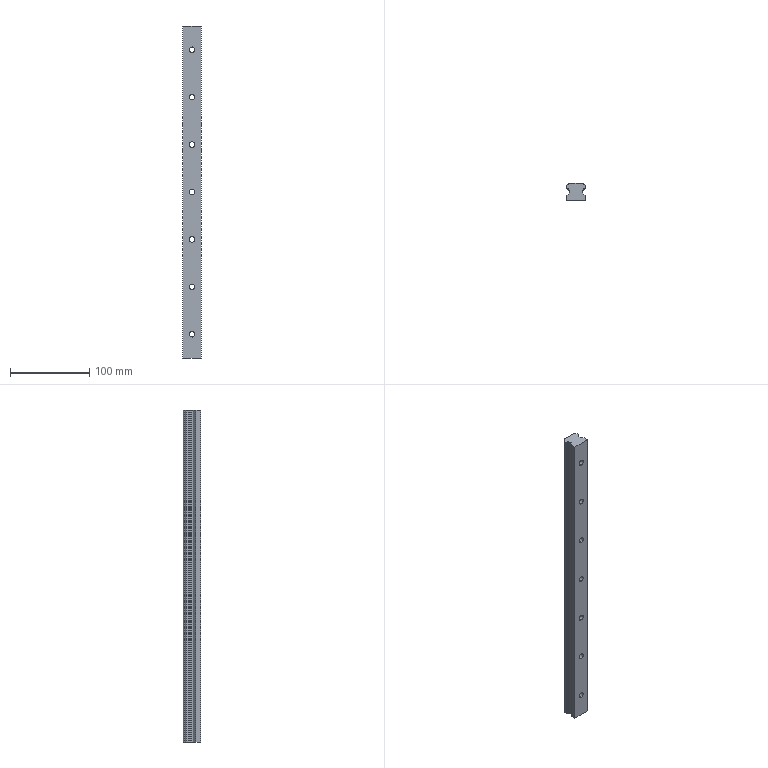Part | SolidWorks | features ICE 17, Chamfer 3, Extrusion 3, Fillet 3, MirrorPattern 3, MirrorSolid 3, RevCut 2, DeleteBody 1, Dome 1, LPattern 1 | 1 solid | 61 faces | box 23 x 22 x 420 mm | volume 180087 mm3 | cylinder 34 | plane 27 | commonest cylinder face diameters 7 x14 11 x14 2.258 x6